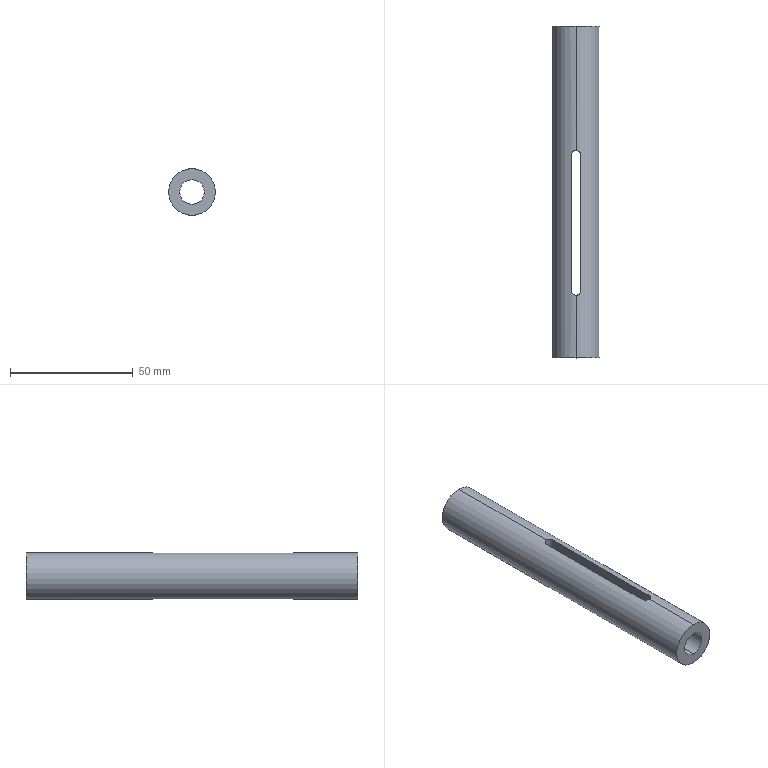Part | STEP file | PN_0063 | 1 solid | 20 faces | box 19 x 135 x 19 mm | volume 21830 mm3 | cylinder 10 | plane 6 | cone 4 | commonest cylinder face diameters 4 x4 10 x2 15.5 x2 19 x2